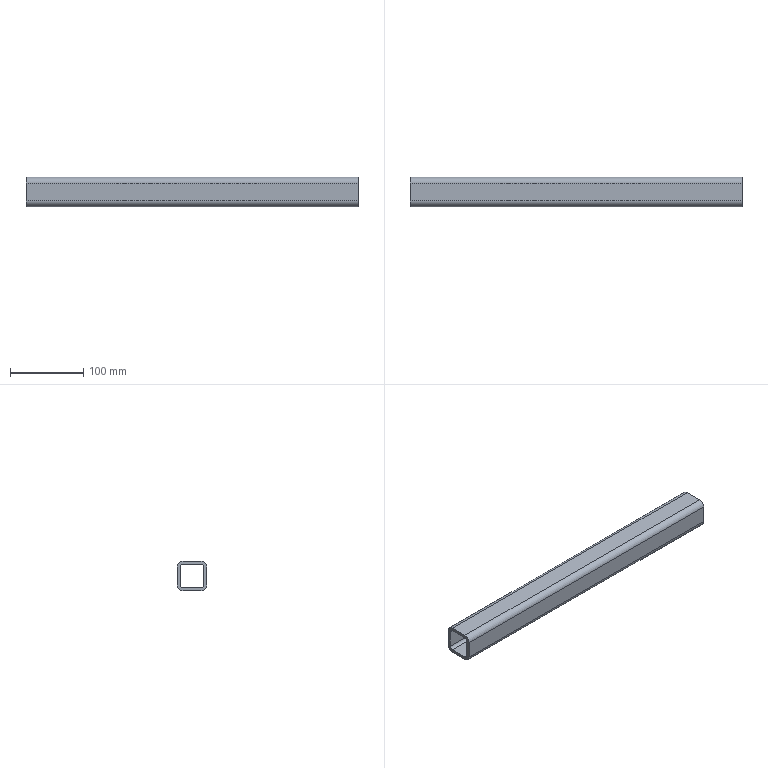Part | STEP file | Flat conveyor mechanism-CN2500x400-105-102_Default<As machined> | 1 solid | 18 faces | box 452 x 40 x 40 mm | volume 241728 mm3 | plane 10 | cylinder 8 | commonest cylinder face diameters 8 x4 16 x4
STEP:
#1=CARTESIAN_POINT('',(0.,-20.,12.));
#2=VERTEX_POINT('',#1);
#3=CARTESIAN_POINT('',(0.,-12.,20.));
#4=VERTEX_POINT('',#3);
#5=CARTESIAN_POINT('',(0.,-12.,12.));
#6=DIRECTION('',(-1.,0.,0.));
#7=DIRECTION('',(0.,-1.,0.));
#8=AXIS2_PLACEMENT_3D('',#5,#6,#7);
#9=CIRCLE('',#8,8.);
#10=EDGE_CURVE('',#2,#4,#9,.T.);
#11=ORIENTED_EDGE('',*,*,#10,.T.);
#12=CARTESIAN_POINT('',(-452.,-12.,20.));
#13=VERTEX_POINT('',#12);
#14=CARTESIAN_POINT('',(-452.,-12.,20.));
#15=DIRECTION('',(1.,0.,0.));
#16=VECTOR('',#15,1000.);
#17=LINE('',#14,#16);
#18=EDGE_CURVE('',#13,#4,#17,.T.);
#19=ORIENTED_EDGE('',*,*,#18,.F.);
#20=CARTESIAN_POINT('',(-452.,-20.,12.));
#21=VERTEX_POINT('',#20);
#22=CARTESIAN_POINT('',(-452.,-12.,12.));
#23=DIRECTION('',(-1.,0.,0.));
#24=DIRECTION('',(0.,-1.,0.));
#25=AXIS2_PLACEMENT_3D('',#22,#23,#24);
#26=CIRCLE('',#25,8.);
#27=EDGE_CURVE('',#21,#13,#26,.T.);
#28=ORIENTED_EDGE('',*,*,#27,.F.);
#29=CARTESIAN_POINT('',(-452.,-20.,12.));
#30=DIRECTION('',(1.,0.,0.));
#31=VECTOR('',#30,1000.);
#32=LINE('',#29,#31);
#33=EDGE_CURVE('',#21,#2,#32,.T.);
#34=ORIENTED_EDGE('',*,*,#33,.T.);
#35=EDGE_LOOP('',(#11,#19,#28,#34));
#36=FACE_OUTER_BOUND('',#35,.T.);
#37=CARTESIAN_POINT('',(-452.,-12.,12.));
#38=DIRECTION('',(1.,0.,0.));
#39=DIRECTION('',(0.,1.,0.));
#40=AXIS2_PLACEMENT_3D('',#37,#38,#39);
#41=CYLINDRICAL_SURFACE('',#40,8.);
#42=ADVANCED_FACE('',(#36),#41,.T.);
#43=CARTESIAN_POINT('',(0.,12.,20.));
#44=VERTEX_POINT('',#43);
#45=CARTESIAN_POINT('',(0.,-12.,20.));
#46=DIRECTION('',(0.,1.,0.));
#47=VECTOR('',#46,1000.);
#48=LINE('',#45,#47);
#49=EDGE_CURVE('',#4,#44,#48,.T.);
#50=ORIENTED_EDGE('',*,*,#49,.T.);
#51=CARTESIAN_POINT('',(-452.,12.,20.));
#52=VERTEX_POINT('',#51);
#53=CARTESIAN_POINT('',(-452.,12.,20.));
#54=DIRECTION('',(1.,0.,0.));
#55=VECTOR('',#54,1000.);
#56=LINE('',#53,#55);
#57=EDGE_CURVE('',#52,#44,#56,.T.);
#58=ORIENTED_EDGE('',*,*,#57,.F.);
#59=CARTESIAN_POINT('',(-452.,-12.,20.));
#60=DIRECTION('',(0.,1.,0.));
#61=VECTOR('',#60,1000.);
#62=LINE('',#59,#61);
#63=EDGE_CURVE('',#13,#52,#62,.T.);
#64=ORIENTED_EDGE('',*,*,#63,.F.);
#65=ORIENTED_EDGE('',*,*,#18,.T.);
#66=EDGE_LOOP('',(#50,#58,#64,#65));
#67=FACE_OUTER_BOUND('',#66,.T.);
#68=CARTESIAN_POINT('',(-452.,-12.,20.));
#69=DIRECTION('',(0.,0.,-1.));
#70=DIRECTION('',(-1.,0.,0.));
#71=AXIS2_PLACEMENT_3D('',#68,#69,#70);
#72=PLANE('',#71);
#73=ADVANCED_FACE('',(#67),#72,.F.);
#74=CARTESIAN_POINT('',(0.,20.,12.));
#75=VERTEX_POINT('',#74);
#76=CARTESIAN_POINT('',(0.,12.,12.));
#77=DIRECTION('',(-1.,0.,0.));
#78=DIRECTION('',(0.,-1.,0.));
#79=AXIS2_PLACEMENT_3D('',#76,#77,#78);
#80=CIRCLE('',#79,8.);
#81=EDGE_CURVE('',#44,#75,#80,.T.);
#82=ORIENTED_EDGE('',*,*,#81,.T.);
#83=CARTESIAN_POINT('',(-452.,20.,12.));
#84=VERTEX_POINT('',#83);
#85=CARTESIAN_POINT('',(-452.,20.,12.));
#86=DIRECTION('',(1.,0.,0.));
#87=VECTOR('',#86,1000.);
#88=LINE('',#85,#87);
#89=EDGE_CURVE('',#84,#75,#88,.T.);
#90=ORIENTED_EDGE('',*,*,#89,.F.);
#91=CARTESIAN_POINT('',(-452.,12.,12.));
#92=DIRECTION('',(-1.,0.,0.));
#93=DIRECTION('',(0.,-1.,0.));
#94=AXIS2_PLACEMENT_3D('',#91,#92,#93);
#95=CIRCLE('',#94,8.);
#96=EDGE_CURVE('',#52,#84,#95,.T.);
#97=ORIENTED_EDGE('',*,*,#96,.F.);
#98=ORIENTED_EDGE('',*,*,#57,.T.);
#99=EDGE_LOOP('',(#82,#90,#97,#98));
#100=FACE_OUTER_BOUND('',#99,.T.);
#101=CARTESIAN_POINT('',(-452.,12.,12.));
#102=DIRECTION('',(1.,0.,0.));
#103=DIRECTION('',(0.,1.,0.));
#104=AXIS2_PLACEMENT_3D('',#101,#102,#103);
#105=CYLINDRICAL_SURFACE('',#104,8.);
#106=ADVANCED_FACE('',(#100),#105,.T.);
#107=CARTESIAN_POINT('',(0.,20.,-12.));
#108=VERTEX_POINT('',#107);
#109=CARTESIAN_POINT('',(0.,20.,-12.));
#110=DIRECTION('',(0.,0.,-1.));
#111=VECTOR('',#110,1000.);
#112=LINE('',#109,#111);
#113=EDGE_CURVE('',#75,#108,#112,.T.);
#114=ORIENTED_EDGE('',*,*,#113,.T.);
#115=CARTESIAN_POINT('',(-452.,20.,-12.));
#116=VERTEX_POINT('',#115);
#117=CARTESIAN_POINT('',(-452.,20.,-12.));
#118=DIRECTION('',(1.,0.,0.));
#119=VECTOR('',#118,1000.);
#120=LINE('',#117,#119);
#121=EDGE_CURVE('',#116,#108,#120,.T.);
#122=ORIENTED_EDGE('',*,*,#121,.F.);
#123=CARTESIAN_POINT('',(-452.,20.,-12.));
#124=DIRECTION('',(0.,0.,-1.));
#125=VECTOR('',#124,1000.);
#126=LINE('',#123,#125);
#127=EDGE_CURVE('',#84,#116,#126,.T.);
#128=ORIENTED_EDGE('',*,*,#127,.F.);
#129=ORIENTED_EDGE('',*,*,#89,.T.);
#130=EDGE_LOOP('',(#114,#122,#128,#129));
#131=FACE_OUTER_BOUND('',#130,.T.);
#132=CARTESIAN_POINT('',(-452.,20.,-12.));
#133=DIRECTION('',(0.,-1.,0.));
#134=DIRECTION('',(1.,0.,0.));
#135=AXIS2_PLACEMENT_3D('',#132,#133,#134);
#136=PLANE('',#135);
#137=ADVANCED_FACE('',(#131),#136,.F.);
#138=CARTESIAN_POINT('',(0.,12.,-20.));
#139=VERTEX_POINT('',#138);
#140=CARTESIAN_POINT('',(0.,12.,-12.));
#141=DIRECTION('',(-1.,0.,0.));
#142=DIRECTION('',(0.,-1.,0.));
#143=AXIS2_PLACEMENT_3D('',#140,#141,#142);
#144=CIRCLE('',#143,8.);
#145=EDGE_CURVE('',#108,#139,#144,.T.);
#146=ORIENTED_EDGE('',*,*,#145,.T.);
#147=CARTESIAN_POINT('',(-452.,12.,-20.));
#148=VERTEX_POINT('',#147);
#149=CARTESIAN_POINT('',(-452.,12.,-20.));
#150=DIRECTION('',(1.,0.,0.));
#151=VECTOR('',#150,1000.);
#152=LINE('',#149,#151);
#153=EDGE_CURVE('',#148,#139,#152,.T.);
#154=ORIENTED_EDGE('',*,*,#153,.F.);
#155=CARTESIAN_POINT('',(-452.,12.,-12.));
#156=DIRECTION('',(-1.,0.,0.));
#157=DIRECTION('',(0.,-1.,0.));
#158=AXIS2_PLACEMENT_3D('',#155,#156,#157);
#159=CIRCLE('',#158,8.);
#160=EDGE_CURVE('',#116,#148,#159,.T.);
#161=ORIENTED_EDGE('',*,*,#160,.F.);
#162=ORIENTED_EDGE('',*,*,#121,.T.);
#163=EDGE_LOOP('',(#146,#154,#161,#162));
#164=FACE_OUTER_BOUND('',#163,.T.);
#165=CARTESIAN_POINT('',(-452.,12.,-12.));
#166=DIRECTION('',(1.,0.,0.));
#167=DIRECTION('',(0.,1.,0.));
#168=AXIS2_PLACEMENT_3D('',#165,#166,#167);
#169=CYLINDRICAL_SURFACE('',#168,8.);
#170=ADVANCED_FACE('',(#164),#169,.T.);
#171=CARTESIAN_POINT('',(0.,-12.,-20.));
#172=VERTEX_POINT('',#171);
#173=CARTESIAN_POINT('',(0.,12.,-20.));
#174=DIRECTION('',(0.,-1.,0.));
#175=VECTOR('',#174,1000.);
#176=LINE('',#173,#175);
#177=EDGE_CURVE('',#139,#172,#176,.T.);
#178=ORIENTED_EDGE('',*,*,#177,.T.);
#179=CARTESIAN_POINT('',(-452.,-12.,-20.));
#180=VERTEX_POINT('',#179);
#181=CARTESIAN_POINT('',(-452.,-12.,-20.));
#182=DIRECTION('',(1.,0.,0.));
#183=VECTOR('',#182,1000.);
#184=LINE('',#181,#183);
#185=EDGE_CURVE('',#180,#172,#184,.T.);
#186=ORIENTED_EDGE('',*,*,#185,.F.);
#187=CARTESIAN_POINT('',(-452.,12.,-20.));
#188=DIRECTION('',(0.,-1.,0.));
#189=VECTOR('',#188,1000.);
#190=LINE('',#187,#189);
#191=EDGE_CURVE('',#148,#180,#190,.T.);
#192=ORIENTED_EDGE('',*,*,#191,.F.);
#193=ORIENTED_EDGE('',*,*,#153,.T.);
#194=EDGE_LOOP('',(#178,#186,#192,#193));
#195=FACE_OUTER_BOUND('',#194,.T.);
#196=CARTESIAN_POINT('',(-452.,12.,-20.));
#197=DIRECTION('',(0.,0.,1.));
#198=DIRECTION('',(1.,0.,0.));
#199=AXIS2_PLACEMENT_3D('',#196,#197,#198);
#200=PLANE('',#199);
#201=ADVANCED_FACE('',(#195),#200,.F.);
#202=CARTESIAN_POINT('',(0.,-20.,-12.));
#203=VERTEX_POINT('',#202);
#204=CARTESIAN_POINT('',(0.,-12.,-12.));
#205=DIRECTION('',(-1.,0.,0.));
#206=DIRECTION('',(0.,-1.,0.));
#207=AXIS2_PLACEMENT_3D('',#204,#205,#206);
#208=CIRCLE('',#207,8.);
#209=EDGE_CURVE('',#172,#203,#208,.T.);
#210=ORIENTED_EDGE('',*,*,#209,.T.);
#211=CARTESIAN_POINT('',(-452.,-20.,-12.));
#212=VERTEX_POINT('',#211);
#213=CARTESIAN_POINT('',(-452.,-20.,-12.));
#214=DIRECTION('',(1.,0.,0.));
#215=VECTOR('',#214,1000.);
#216=LINE('',#213,#215);
#217=EDGE_CURVE('',#212,#203,#216,.T.);
#218=ORIENTED_EDGE('',*,*,#217,.F.);
#219=CARTESIAN_POINT('',(-452.,-12.,-12.));
#220=DIRECTION('',(-1.,0.,0.));
#221=DIRECTION('',(0.,-1.,0.));
#222=AXIS2_PLACEMENT_3D('',#219,#220,#221);
#223=CIRCLE('',#222,8.);
#224=EDGE_CURVE('',#180,#212,#223,.T.);
#225=ORIENTED_EDGE('',*,*,#224,.F.);
#226=ORIENTED_EDGE('',*,*,#185,.T.);
#227=EDGE_LOOP('',(#210,#218,#225,#226));
#228=FACE_OUTER_BOUND('',#227,.T.);
#229=CARTESIAN_POINT('',(-452.,-12.,-12.));
#230=DIRECTION('',(1.,0.,0.));
#231=DIRECTION('',(0.,1.,0.));
#232=AXIS2_PLACEMENT_3D('',#229,#230,#231);
#233=CYLINDRICAL_SURFACE('',#232,8.);
#234=ADVANCED_FACE('',(#228),#233,.T.);
#235=CARTESIAN_POINT('',(0.,12.,16.));
#236=VERTEX_POINT('',#235);
#237=CARTESIAN_POINT('',(0.,16.,12.));
#238=VERTEX_POINT('',#237);
#239=CARTESIAN_POINT('',(0.,12.,12.));
#240=DIRECTION('',(-1.,0.,0.));
#241=DIRECTION('',(0.,-1.,0.));
#242=AXIS2_PLACEMENT_3D('',#239,#240,#241);
#243=CIRCLE('',#242,4.);
#244=EDGE_CURVE('',#236,#238,#243,.T.);
#245=ORIENTED_EDGE('',*,*,#244,.F.);
#246=CARTESIAN_POINT('',(-452.,12.,16.));
#247=VERTEX_POINT('',#246);
#248=CARTESIAN_POINT('',(-452.,12.,16.));
#249=DIRECTION('',(1.,0.,0.));
#250=VECTOR('',#249,1000.);
#251=LINE('',#248,#250);
#252=EDGE_CURVE('',#247,#236,#251,.T.);
#253=ORIENTED_EDGE('',*,*,#252,.F.);
#254=CARTESIAN_POINT('',(-452.,16.,12.));
#255=VERTEX_POINT('',#254);
#256=CARTESIAN_POINT('',(-452.,12.,12.));
#257=DIRECTION('',(-1.,0.,0.));
#258=DIRECTION('',(0.,-1.,0.));
#259=AXIS2_PLACEMENT_3D('',#256,#257,#258);
#260=CIRCLE('',#259,4.);
#261=EDGE_CURVE('',#247,#255,#260,.T.);
#262=ORIENTED_EDGE('',*,*,#261,.T.);
#263=CARTESIAN_POINT('',(-452.,16.,12.));
#264=DIRECTION('',(1.,0.,0.));
#265=VECTOR('',#264,1000.);
#266=LINE('',#263,#265);
#267=EDGE_CURVE('',#255,#238,#266,.T.);
#268=ORIENTED_EDGE('',*,*,#267,.T.);
#269=EDGE_LOOP('',(#245,#253,#262,#268));
#270=FACE_OUTER_BOUND('',#269,.T.);
#271=CARTESIAN_POINT('',(-452.,12.,12.));
#272=DIRECTION('',(1.,0.,0.));
#273=DIRECTION('',(0.,1.,0.));
#274=AXIS2_PLACEMENT_3D('',#271,#272,#273);
#275=CYLINDRICAL_SURFACE('',#274,4.);
#276=ADVANCED_FACE('',(#270),#275,.F.);
#277=CARTESIAN_POINT('',(0.,-12.,16.));
#278=VERTEX_POINT('',#277);
#279=CARTESIAN_POINT('',(0.,-12.,16.));
#280=DIRECTION('',(0.,1.,0.));
#281=VECTOR('',#280,1000.);
#282=LINE('',#279,#281);
#283=EDGE_CURVE('',#278,#236,#282,.T.);
#284=ORIENTED_EDGE('',*,*,#283,.F.);
#285=CARTESIAN_POINT('',(-452.,-12.,16.));
#286=VERTEX_POINT('',#285);
#287=CARTESIAN_POINT('',(-452.,-12.,16.));
#288=DIRECTION('',(1.,0.,0.));
#289=VECTOR('',#288,1000.);
#290=LINE('',#287,#289);
#291=EDGE_CURVE('',#286,#278,#290,.T.);
#292=ORIENTED_EDGE('',*,*,#291,.F.);
#293=CARTESIAN_POINT('',(-452.,-12.,16.));
#294=DIRECTION('',(0.,1.,0.));
#295=VECTOR('',#294,1000.);
#296=LINE('',#293,#295);
#297=EDGE_CURVE('',#286,#247,#296,.T.);
#298=ORIENTED_EDGE('',*,*,#297,.T.);
#299=ORIENTED_EDGE('',*,*,#252,.T.);
#300=EDGE_LOOP('',(#284,#292,#298,#299));
#301=FACE_OUTER_BOUND('',#300,.T.);
#302=CARTESIAN_POINT('',(-452.,-12.,16.));
#303=DIRECTION('',(0.,0.,-1.));
#304=DIRECTION('',(-1.,0.,0.));
#305=AXIS2_PLACEMENT_3D('',#302,#303,#304);
#306=PLANE('',#305);
#307=ADVANCED_FACE('',(#301),#306,.T.);
#308=CARTESIAN_POINT('',(0.,-16.,12.));
#309=VERTEX_POINT('',#308);
#310=CARTESIAN_POINT('',(0.,-12.,12.));
#311=DIRECTION('',(-1.,0.,0.));
#312=DIRECTION('',(0.,-1.,0.));
#313=AXIS2_PLACEMENT_3D('',#310,#311,#312);
#314=CIRCLE('',#313,4.);
#315=EDGE_CURVE('',#309,#278,#314,.T.);
#316=ORIENTED_EDGE('',*,*,#315,.F.);
#317=CARTESIAN_POINT('',(-452.,-16.,12.));
#318=VERTEX_POINT('',#317);
#319=CARTESIAN_POINT('',(-452.,-16.,12.));
#320=DIRECTION('',(1.,0.,0.));
#321=VECTOR('',#320,1000.);
#322=LINE('',#319,#321);
#323=EDGE_CURVE('',#318,#309,#322,.T.);
#324=ORIENTED_EDGE('',*,*,#323,.F.);
#325=CARTESIAN_POINT('',(-452.,-12.,12.));
#326=DIRECTION('',(-1.,0.,0.));
#327=DIRECTION('',(0.,-1.,0.));
#328=AXIS2_PLACEMENT_3D('',#325,#326,#327);
#329=CIRCLE('',#328,4.);
#330=EDGE_CURVE('',#318,#286,#329,.T.);
#331=ORIENTED_EDGE('',*,*,#330,.T.);
#332=ORIENTED_EDGE('',*,*,#291,.T.);
#333=EDGE_LOOP('',(#316,#324,#331,#332));
#334=FACE_OUTER_BOUND('',#333,.T.);
#335=CARTESIAN_POINT('',(-452.,-12.,12.));
#336=DIRECTION('',(1.,0.,0.));
#337=DIRECTION('',(0.,1.,0.));
#338=AXIS2_PLACEMENT_3D('',#335,#336,#337);
#339=CYLINDRICAL_SURFACE('',#338,4.);
#340=ADVANCED_FACE('',(#334),#339,.F.);
#341=CARTESIAN_POINT('',(0.,-16.,-12.));
#342=VERTEX_POINT('',#341);
#343=CARTESIAN_POINT('',(0.,-16.,12.));
#344=DIRECTION('',(0.,0.,1.));
#345=VECTOR('',#344,1000.);
#346=LINE('',#343,#345);
#347=EDGE_CURVE('',#342,#309,#346,.T.);
#348=ORIENTED_EDGE('',*,*,#347,.F.);
#349=CARTESIAN_POINT('',(-452.,-16.,-12.));
#350=VERTEX_POINT('',#349);
#351=CARTESIAN_POINT('',(-452.,-16.,-12.));
#352=DIRECTION('',(1.,0.,0.));
#353=VECTOR('',#352,1000.);
#354=LINE('',#351,#353);
#355=EDGE_CURVE('',#350,#342,#354,.T.);
#356=ORIENTED_EDGE('',*,*,#355,.F.);
#357=CARTESIAN_POINT('',(-452.,-16.,12.));
#358=DIRECTION('',(0.,0.,1.));
#359=VECTOR('',#358,1000.);
#360=LINE('',#357,#359);
#361=EDGE_CURVE('',#350,#318,#360,.T.);
#362=ORIENTED_EDGE('',*,*,#361,.T.);
#363=ORIENTED_EDGE('',*,*,#323,.T.);
#364=EDGE_LOOP('',(#348,#356,#362,#363));
#365=FACE_OUTER_BOUND('',#364,.T.);
#366=CARTESIAN_POINT('',(-452.,-16.,12.));
#367=DIRECTION('',(0.,1.,0.));
#368=DIRECTION('',(-1.,0.,0.));
#369=AXIS2_PLACEMENT_3D('',#366,#367,#368);
#370=PLANE('',#369);
#371=ADVANCED_FACE('',(#365),#370,.T.);
#372=CARTESIAN_POINT('',(0.,-12.,-16.));
#373=VERTEX_POINT('',#372);
#374=CARTESIAN_POINT('',(0.,-12.,-12.));
#375=DIRECTION('',(-1.,0.,0.));
#376=DIRECTION('',(0.,-1.,0.));
#377=AXIS2_PLACEMENT_3D('',#374,#375,#376);
#378=CIRCLE('',#377,4.);
#379=EDGE_CURVE('',#373,#342,#378,.T.);
#380=ORIENTED_EDGE('',*,*,#379,.F.);
#381=CARTESIAN_POINT('',(-452.,-12.,-16.));
#382=VERTEX_POINT('',#381);
#383=CARTESIAN_POINT('',(-452.,-12.,-16.));
#384=DIRECTION('',(1.,0.,0.));
#385=VECTOR('',#384,1000.);
#386=LINE('',#383,#385);
#387=EDGE_CURVE('',#382,#373,#386,.T.);
#388=ORIENTED_EDGE('',*,*,#387,.F.);
#389=CARTESIAN_POINT('',(-452.,-12.,-12.));
#390=DIRECTION('',(-1.,0.,0.));
#391=DIRECTION('',(0.,-1.,0.));
#392=AXIS2_PLACEMENT_3D('',#389,#390,#391);
#393=CIRCLE('',#392,4.);
#394=EDGE_CURVE('',#382,#350,#393,.T.);
#395=ORIENTED_EDGE('',*,*,#394,.T.);
#396=ORIENTED_EDGE('',*,*,#355,.T.);
#397=EDGE_LOOP('',(#380,#388,#395,#396));
#398=FACE_OUTER_BOUND('',#397,.T.);
#399=CARTESIAN_POINT('',(-452.,-12.,-12.));
#400=DIRECTION('',(1.,0.,0.));
#401=DIRECTION('',(0.,1.,0.));
#402=AXIS2_PLACEMENT_3D('',#399,#400,#401);
#403=CYLINDRICAL_SURFACE('',#402,4.);
#404=ADVANCED_FACE('',(#398),#403,.F.);
#405=CARTESIAN_POINT('',(0.,12.,-16.));
#406=VERTEX_POINT('',#405);
#407=CARTESIAN_POINT('',(0.,12.,-16.));
#408=DIRECTION('',(0.,-1.,0.));
#409=VECTOR('',#408,1000.);
#410=LINE('',#407,#409);
#411=EDGE_CURVE('',#406,#373,#410,.T.);
#412=ORIENTED_EDGE('',*,*,#411,.F.);
#413=CARTESIAN_POINT('',(-452.,12.,-16.));
#414=VERTEX_POINT('',#413);
#415=CARTESIAN_POINT('',(-452.,12.,-16.));
#416=DIRECTION('',(1.,0.,0.));
#417=VECTOR('',#416,1000.);
#418=LINE('',#415,#417);
#419=EDGE_CURVE('',#414,#406,#418,.T.);
#420=ORIENTED_EDGE('',*,*,#419,.F.);
#421=CARTESIAN_POINT('',(-452.,12.,-16.));
#422=DIRECTION('',(0.,-1.,0.));
#423=VECTOR('',#422,1000.);
#424=LINE('',#421,#423);
#425=EDGE_CURVE('',#414,#382,#424,.T.);
#426=ORIENTED_EDGE('',*,*,#425,.T.);
#427=ORIENTED_EDGE('',*,*,#387,.T.);
#428=EDGE_LOOP('',(#412,#420,#426,#427));
#429=FACE_OUTER_BOUND('',#428,.T.);
#430=CARTESIAN_POINT('',(-452.,12.,-16.));
#431=DIRECTION('',(0.,0.,1.));
#432=DIRECTION('',(1.,0.,0.));
#433=AXIS2_PLACEMENT_3D('',#430,#431,#432);
#434=PLANE('',#433);
#435=ADVANCED_FACE('',(#429),#434,.T.);
#436=CARTESIAN_POINT('',(0.,16.,-12.));
#437=VERTEX_POINT('',#436);
#438=CARTESIAN_POINT('',(0.,12.,-12.));
#439=DIRECTION('',(-1.,0.,0.));
#440=DIRECTION('',(0.,-1.,0.));
#441=AXIS2_PLACEMENT_3D('',#438,#439,#440);
#442=CIRCLE('',#441,4.);
#443=EDGE_CURVE('',#437,#406,#442,.T.);
#444=ORIENTED_EDGE('',*,*,#443,.F.);
#445=CARTESIAN_POINT('',(-452.,16.,-12.));
#446=VERTEX_POINT('',#445);
#447=CARTESIAN_POINT('',(-452.,16.,-12.));
#448=DIRECTION('',(1.,0.,0.));
#449=VECTOR('',#448,1000.);
#450=LINE('',#447,#449);
#451=EDGE_CURVE('',#446,#437,#450,.T.);
#452=ORIENTED_EDGE('',*,*,#451,.F.);
#453=CARTESIAN_POINT('',(-452.,12.,-12.));
#454=DIRECTION('',(-1.,0.,0.));
#455=DIRECTION('',(0.,-1.,0.));
#456=AXIS2_PLACEMENT_3D('',#453,#454,#455);
#457=CIRCLE('',#456,4.);
#458=EDGE_CURVE('',#446,#414,#457,.T.);
#459=ORIENTED_EDGE('',*,*,#458,.T.);
#460=ORIENTED_EDGE('',*,*,#419,.T.);
#461=EDGE_LOOP('',(#444,#452,#459,#460));
#462=FACE_OUTER_BOUND('',#461,.T.);
#463=CARTESIAN_POINT('',(-452.,12.,-12.));
#464=DIRECTION('',(1.,0.,0.));
#465=DIRECTION('',(0.,1.,0.));
#466=AXIS2_PLACEMENT_3D('',#463,#464,#465);
#467=CYLINDRICAL_SURFACE('',#466,4.);
#468=ADVANCED_FACE('',(#462),#467,.F.);
#469=CARTESIAN_POINT('',(0.,16.,-12.));
#470=DIRECTION('',(0.,0.,-1.));
#471=VECTOR('',#470,1000.);
#472=LINE('',#469,#471);
#473=EDGE_CURVE('',#238,#437,#472,.T.);
#474=ORIENTED_EDGE('',*,*,#473,.F.);
#475=ORIENTED_EDGE('',*,*,#267,.F.);
#476=CARTESIAN_POINT('',(-452.,16.,-12.));
#477=DIRECTION('',(0.,0.,-1.));
#478=VECTOR('',#477,1000.);
#479=LINE('',#476,#478);
#480=EDGE_CURVE('',#255,#446,#479,.T.);
#481=ORIENTED_EDGE('',*,*,#480,.T.);
#482=ORIENTED_EDGE('',*,*,#451,.T.);
#483=EDGE_LOOP('',(#474,#475,#481,#482));
#484=FACE_OUTER_BOUND('',#483,.T.);
#485=CARTESIAN_POINT('',(-452.,16.,-12.));
#486=DIRECTION('',(0.,-1.,0.));
#487=DIRECTION('',(1.,0.,0.));
#488=AXIS2_PLACEMENT_3D('',#485,#486,#487);
#489=PLANE('',#488);
#490=ADVANCED_FACE('',(#484),#489,.T.);
#491=CARTESIAN_POINT('',(0.,-20.,12.));
#492=DIRECTION('',(0.,0.,1.));
#493=VECTOR('',#492,1000.);
#494=LINE('',#491,#493);
#495=EDGE_CURVE('',#203,#2,#494,.T.);
#496=ORIENTED_EDGE('',*,*,#495,.T.);
#497=ORIENTED_EDGE('',*,*,#33,.F.);
#498=CARTESIAN_POINT('',(-452.,-20.,12.));
#499=DIRECTION('',(0.,0.,1.));
#500=VECTOR('',#499,1000.);
#501=LINE('',#498,#500);
#502=EDGE_CURVE('',#212,#21,#501,.T.);
#503=ORIENTED_EDGE('',*,*,#502,.F.);
#504=ORIENTED_EDGE('',*,*,#217,.T.);
#505=EDGE_LOOP('',(#496,#497,#503,#504));
#506=FACE_OUTER_BOUND('',#505,.T.);
#507=CARTESIAN_POINT('',(-452.,-20.,12.));
#508=DIRECTION('',(0.,1.,0.));
#509=DIRECTION('',(-1.,0.,0.));
#510=AXIS2_PLACEMENT_3D('',#507,#508,#509);
#511=PLANE('',#510);
#512=ADVANCED_FACE('',(#506),#511,.F.);
#513=ORIENTED_EDGE('',*,*,#261,.F.);
#514=ORIENTED_EDGE('',*,*,#297,.F.);
#515=ORIENTED_EDGE('',*,*,#330,.F.);
#516=ORIENTED_EDGE('',*,*,#361,.F.);
#517=ORIENTED_EDGE('',*,*,#394,.F.);
#518=ORIENTED_EDGE('',*,*,#425,.F.);
#519=ORIENTED_EDGE('',*,*,#458,.F.);
#520=ORIENTED_EDGE('',*,*,#480,.F.);
#521=EDGE_LOOP('',(#513,#514,#515,#516,#517,#518,#519,#520));
#522=FACE_BOUND('',#521,.T.);
#523=ORIENTED_EDGE('',*,*,#27,.T.);
#524=ORIENTED_EDGE('',*,*,#63,.T.);
#525=ORIENTED_EDGE('',*,*,#96,.T.);
#526=ORIENTED_EDGE('',*,*,#127,.T.);
#527=ORIENTED_EDGE('',*,*,#160,.T.);
#528=ORIENTED_EDGE('',*,*,#191,.T.);
#529=ORIENTED_EDGE('',*,*,#224,.T.);
#530=ORIENTED_EDGE('',*,*,#502,.T.);
#531=EDGE_LOOP('',(#523,#524,#525,#526,#527,#528,#529,#530));
#532=FACE_OUTER_BOUND('',#531,.T.);
#533=CARTESIAN_POINT('',(-452.,-12.,12.));
#534=DIRECTION('',(-1.,0.,0.));
#535=DIRECTION('',(0.,-1.,0.));
#536=AXIS2_PLACEMENT_3D('',#533,#534,#535);
#537=PLANE('',#536);
#538=ADVANCED_FACE('',(#522,#532),#537,.T.);
#539=ORIENTED_EDGE('',*,*,#244,.T.);
#540=ORIENTED_EDGE('',*,*,#473,.T.);
#541=ORIENTED_EDGE('',*,*,#443,.T.);
#542=ORIENTED_EDGE('',*,*,#411,.T.);
#543=ORIENTED_EDGE('',*,*,#379,.T.);
#544=ORIENTED_EDGE('',*,*,#347,.T.);
#545=ORIENTED_EDGE('',*,*,#315,.T.);
#546=ORIENTED_EDGE('',*,*,#283,.T.);
#547=EDGE_LOOP('',(#539,#540,#541,#542,#543,#544,#545,#546));
#548=FACE_BOUND('',#547,.T.);
#549=ORIENTED_EDGE('',*,*,#10,.F.);
#550=ORIENTED_EDGE('',*,*,#495,.F.);
#551=ORIENTED_EDGE('',*,*,#209,.F.);
#552=ORIENTED_EDGE('',*,*,#177,.F.);
#553=ORIENTED_EDGE('',*,*,#145,.F.);
#554=ORIENTED_EDGE('',*,*,#113,.F.);
#555=ORIENTED_EDGE('',*,*,#81,.F.);
#556=ORIENTED_EDGE('',*,*,#49,.F.);
#557=EDGE_LOOP('',(#549,#550,#551,#552,#553,#554,#555,#556));
#558=FACE_OUTER_BOUND('',#557,.T.);
#559=CARTESIAN_POINT('',(0.,-12.,12.));
#560=DIRECTION('',(-1.,0.,0.));
#561=DIRECTION('',(0.,-1.,0.));
#562=AXIS2_PLACEMENT_3D('',#559,#560,#561);
#563=PLANE('',#562);
#564=ADVANCED_FACE('',(#548,#558),#563,.F.);
#565=CLOSED_SHELL('',(#42,#73,#106,#137,#170,#201,#234,#276,#307,#340,#371,#404,#435,#468,#490,#512,#538,#564));
#566=MANIFOLD_SOLID_BREP('',#565);
#567=CARTESIAN_POINT('',(0.,0.,0.));
#568=DIRECTION('',(0.,0.,1.));
#569=DIRECTION('',(1.,0.,0.));
#570=AXIS2_PLACEMENT_3D('',#567,#568,#569);
#571=(LENGTH_UNIT()NAMED_UNIT(*)SI_UNIT(.MILLI.,.METRE.));
#572=UNCERTAINTY_MEASURE_WITH_UNIT(LENGTH_MEASURE(0.00001),#571,'','');
#573=(NAMED_UNIT(*)PLANE_ANGLE_UNIT()SI_UNIT($,.RADIAN.));
#574=(NAMED_UNIT(*)SI_UNIT($,.STERADIAN.)SOLID_ANGLE_UNIT());
#575=(GEOMETRIC_REPRESENTATION_CONTEXT(3)GLOBAL_UNCERTAINTY_ASSIGNED_CONTEXT((#572))GLOBAL_UNIT_ASSIGNED_CONTEXT((#571,#573,#574))REPRESENTATION_CONTEXT('',''));
#576=ADVANCED_BREP_SHAPE_REPRESENTATION('',(#566,#570),#575);